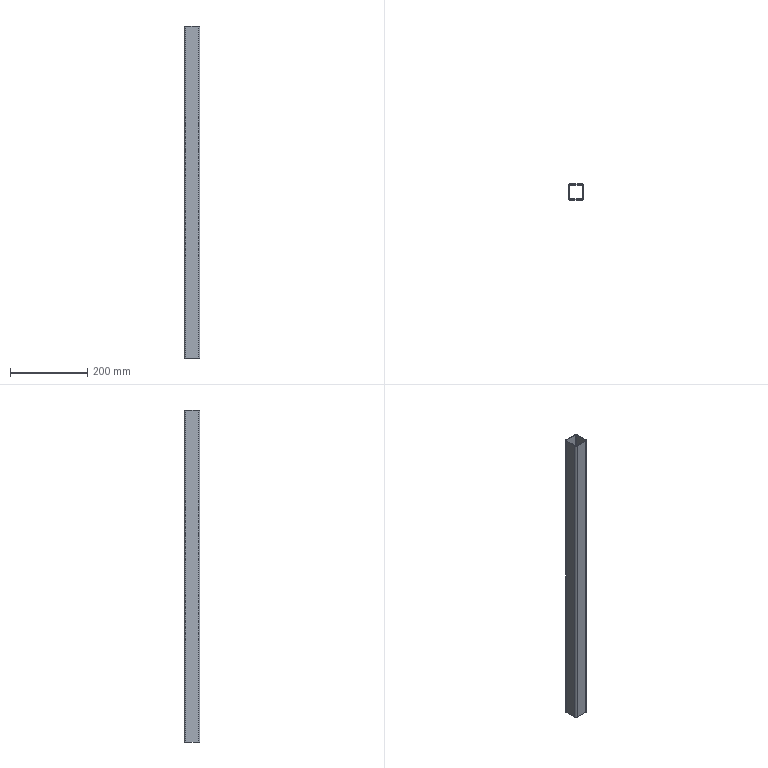Part | SolidWorks | features Fillet 2, Extrusion 1 | 1 solid | 18 faces | box 40 x 40 x 860 mm | volume 252581 mm3 | plane 10 | cylinder 8 | commonest cylinder face diameters 4 x4 8 x4
STEP:
#1=CARTESIAN_POINT('',(20.,-16.,860.));
#2=VERTEX_POINT('',#1);
#3=CARTESIAN_POINT('',(20.,16.,860.));
#4=VERTEX_POINT('',#3);
#5=CARTESIAN_POINT('',(20.,20.,860.));
#6=DIRECTION('',(0.,1.,0.));
#7=VECTOR('',#6,1000.);
#8=LINE('',#5,#7);
#9=EDGE_CURVE('',#2,#4,#8,.T.);
#10=ORIENTED_EDGE('',*,*,#9,.T.);
#11=CARTESIAN_POINT('',(16.,20.,860.));
#12=VERTEX_POINT('',#11);
#13=CARTESIAN_POINT('',(16.,16.,860.));
#14=DIRECTION('',(0.,0.,1.));
#15=DIRECTION('',(1.,0.,0.));
#16=AXIS2_PLACEMENT_3D('',#13,#14,#15);
#17=CIRCLE('',#16,4.);
#18=EDGE_CURVE('',#4,#12,#17,.T.);
#19=ORIENTED_EDGE('',*,*,#18,.T.);
#20=CARTESIAN_POINT('',(-16.,20.,860.));
#21=VERTEX_POINT('',#20);
#22=CARTESIAN_POINT('',(-20.,20.,860.));
#23=DIRECTION('',(-1.,0.,0.));
#24=VECTOR('',#23,1000.);
#25=LINE('',#22,#24);
#26=EDGE_CURVE('',#12,#21,#25,.T.);
#27=ORIENTED_EDGE('',*,*,#26,.T.);
#28=CARTESIAN_POINT('',(-20.,16.,860.));
#29=VERTEX_POINT('',#28);
#30=CARTESIAN_POINT('',(-16.,16.,860.));
#31=DIRECTION('',(0.,0.,1.));
#32=DIRECTION('',(1.,0.,0.));
#33=AXIS2_PLACEMENT_3D('',#30,#31,#32);
#34=CIRCLE('',#33,4.);
#35=EDGE_CURVE('',#21,#29,#34,.T.);
#36=ORIENTED_EDGE('',*,*,#35,.T.);
#37=CARTESIAN_POINT('',(-20.,-16.,860.));
#38=VERTEX_POINT('',#37);
#39=CARTESIAN_POINT('',(-20.,20.,860.));
#40=DIRECTION('',(0.,-1.,0.));
#41=VECTOR('',#40,1000.);
#42=LINE('',#39,#41);
#43=EDGE_CURVE('',#29,#38,#42,.T.);
#44=ORIENTED_EDGE('',*,*,#43,.T.);
#45=CARTESIAN_POINT('',(-16.,-20.,860.));
#46=VERTEX_POINT('',#45);
#47=CARTESIAN_POINT('',(-16.,-16.,860.));
#48=DIRECTION('',(0.,0.,1.));
#49=DIRECTION('',(1.,0.,0.));
#50=AXIS2_PLACEMENT_3D('',#47,#48,#49);
#51=CIRCLE('',#50,4.);
#52=EDGE_CURVE('',#38,#46,#51,.T.);
#53=ORIENTED_EDGE('',*,*,#52,.T.);
#54=CARTESIAN_POINT('',(16.,-20.,860.));
#55=VERTEX_POINT('',#54);
#56=CARTESIAN_POINT('',(-20.,-20.,860.));
#57=DIRECTION('',(1.,0.,0.));
#58=VECTOR('',#57,1000.);
#59=LINE('',#56,#58);
#60=EDGE_CURVE('',#46,#55,#59,.T.);
#61=ORIENTED_EDGE('',*,*,#60,.T.);
#62=CARTESIAN_POINT('',(16.,-16.,860.));
#63=DIRECTION('',(0.,0.,1.));
#64=DIRECTION('',(1.,0.,0.));
#65=AXIS2_PLACEMENT_3D('',#62,#63,#64);
#66=CIRCLE('',#65,4.);
#67=EDGE_CURVE('',#55,#2,#66,.T.);
#68=ORIENTED_EDGE('',*,*,#67,.T.);
#69=EDGE_LOOP('',(#10,#19,#27,#36,#44,#53,#61,#68));
#70=FACE_OUTER_BOUND('',#69,.T.);
#71=CARTESIAN_POINT('',(16.,18.,860.));
#72=VERTEX_POINT('',#71);
#73=CARTESIAN_POINT('',(-16.,18.,860.));
#74=VERTEX_POINT('',#73);
#75=CARTESIAN_POINT('',(-18.,18.,860.));
#76=DIRECTION('',(-1.,0.,0.));
#77=VECTOR('',#76,1000.);
#78=LINE('',#75,#77);
#79=EDGE_CURVE('',#72,#74,#78,.T.);
#80=ORIENTED_EDGE('',*,*,#79,.F.);
#81=CARTESIAN_POINT('',(18.,16.,860.));
#82=VERTEX_POINT('',#81);
#83=CARTESIAN_POINT('',(16.,16.,860.));
#84=DIRECTION('',(0.,0.,-1.));
#85=DIRECTION('',(1.,0.,0.));
#86=AXIS2_PLACEMENT_3D('',#83,#84,#85);
#87=CIRCLE('',#86,2.);
#88=EDGE_CURVE('',#72,#82,#87,.T.);
#89=ORIENTED_EDGE('',*,*,#88,.T.);
#90=CARTESIAN_POINT('',(18.,-16.,860.));
#91=VERTEX_POINT('',#90);
#92=CARTESIAN_POINT('',(18.,18.,860.));
#93=DIRECTION('',(0.,1.,0.));
#94=VECTOR('',#93,1000.);
#95=LINE('',#92,#94);
#96=EDGE_CURVE('',#91,#82,#95,.T.);
#97=ORIENTED_EDGE('',*,*,#96,.F.);
#98=CARTESIAN_POINT('',(16.,-18.,860.));
#99=VERTEX_POINT('',#98);
#100=CARTESIAN_POINT('',(16.,-16.,860.));
#101=DIRECTION('',(0.,0.,-1.));
#102=DIRECTION('',(1.,0.,0.));
#103=AXIS2_PLACEMENT_3D('',#100,#101,#102);
#104=CIRCLE('',#103,2.);
#105=EDGE_CURVE('',#91,#99,#104,.T.);
#106=ORIENTED_EDGE('',*,*,#105,.T.);
#107=CARTESIAN_POINT('',(-16.,-18.,860.));
#108=VERTEX_POINT('',#107);
#109=CARTESIAN_POINT('',(-18.,-18.,860.));
#110=DIRECTION('',(1.,0.,0.));
#111=VECTOR('',#110,1000.);
#112=LINE('',#109,#111);
#113=EDGE_CURVE('',#108,#99,#112,.T.);
#114=ORIENTED_EDGE('',*,*,#113,.F.);
#115=CARTESIAN_POINT('',(-18.,-16.,860.));
#116=VERTEX_POINT('',#115);
#117=CARTESIAN_POINT('',(-16.,-16.,860.));
#118=DIRECTION('',(0.,0.,-1.));
#119=DIRECTION('',(1.,0.,0.));
#120=AXIS2_PLACEMENT_3D('',#117,#118,#119);
#121=CIRCLE('',#120,2.);
#122=EDGE_CURVE('',#108,#116,#121,.T.);
#123=ORIENTED_EDGE('',*,*,#122,.T.);
#124=CARTESIAN_POINT('',(-18.,16.,860.));
#125=VERTEX_POINT('',#124);
#126=CARTESIAN_POINT('',(-18.,18.,860.));
#127=DIRECTION('',(0.,-1.,0.));
#128=VECTOR('',#127,1000.);
#129=LINE('',#126,#128);
#130=EDGE_CURVE('',#125,#116,#129,.T.);
#131=ORIENTED_EDGE('',*,*,#130,.F.);
#132=CARTESIAN_POINT('',(-16.,16.,860.));
#133=DIRECTION('',(0.,0.,-1.));
#134=DIRECTION('',(1.,0.,0.));
#135=AXIS2_PLACEMENT_3D('',#132,#133,#134);
#136=CIRCLE('',#135,2.);
#137=EDGE_CURVE('',#125,#74,#136,.T.);
#138=ORIENTED_EDGE('',*,*,#137,.T.);
#139=EDGE_LOOP('',(#80,#89,#97,#106,#114,#123,#131,#138));
#140=FACE_BOUND('',#139,.T.);
#141=CARTESIAN_POINT('',(0.,0.,860.));
#142=DIRECTION('',(0.,0.,1.));
#143=DIRECTION('',(1.,0.,0.));
#144=AXIS2_PLACEMENT_3D('',#141,#142,#143);
#145=PLANE('',#144);
#146=ADVANCED_FACE('',(#70,#140),#145,.T.);
#147=CARTESIAN_POINT('',(16.,20.,0.));
#148=VERTEX_POINT('',#147);
#149=CARTESIAN_POINT('',(-16.,20.,0.));
#150=VERTEX_POINT('',#149);
#151=CARTESIAN_POINT('',(-20.,20.,0.));
#152=DIRECTION('',(-1.,0.,0.));
#153=VECTOR('',#152,1000.);
#154=LINE('',#151,#153);
#155=EDGE_CURVE('',#148,#150,#154,.T.);
#156=ORIENTED_EDGE('',*,*,#155,.F.);
#157=CARTESIAN_POINT('',(20.,16.,0.));
#158=VERTEX_POINT('',#157);
#159=CARTESIAN_POINT('',(16.,16.,0.));
#160=DIRECTION('',(0.,0.,-1.));
#161=DIRECTION('',(1.,0.,0.));
#162=AXIS2_PLACEMENT_3D('',#159,#160,#161);
#163=CIRCLE('',#162,4.);
#164=EDGE_CURVE('',#148,#158,#163,.T.);
#165=ORIENTED_EDGE('',*,*,#164,.T.);
#166=CARTESIAN_POINT('',(20.,-16.,0.));
#167=VERTEX_POINT('',#166);
#168=CARTESIAN_POINT('',(20.,20.,0.));
#169=DIRECTION('',(0.,1.,0.));
#170=VECTOR('',#169,1000.);
#171=LINE('',#168,#170);
#172=EDGE_CURVE('',#167,#158,#171,.T.);
#173=ORIENTED_EDGE('',*,*,#172,.F.);
#174=CARTESIAN_POINT('',(16.,-20.,0.));
#175=VERTEX_POINT('',#174);
#176=CARTESIAN_POINT('',(16.,-16.,0.));
#177=DIRECTION('',(0.,0.,-1.));
#178=DIRECTION('',(1.,0.,0.));
#179=AXIS2_PLACEMENT_3D('',#176,#177,#178);
#180=CIRCLE('',#179,4.);
#181=EDGE_CURVE('',#167,#175,#180,.T.);
#182=ORIENTED_EDGE('',*,*,#181,.T.);
#183=CARTESIAN_POINT('',(-16.,-20.,0.));
#184=VERTEX_POINT('',#183);
#185=CARTESIAN_POINT('',(-20.,-20.,0.));
#186=DIRECTION('',(1.,0.,0.));
#187=VECTOR('',#186,1000.);
#188=LINE('',#185,#187);
#189=EDGE_CURVE('',#184,#175,#188,.T.);
#190=ORIENTED_EDGE('',*,*,#189,.F.);
#191=CARTESIAN_POINT('',(-20.,-16.,0.));
#192=VERTEX_POINT('',#191);
#193=CARTESIAN_POINT('',(-16.,-16.,0.));
#194=DIRECTION('',(0.,0.,-1.));
#195=DIRECTION('',(1.,0.,0.));
#196=AXIS2_PLACEMENT_3D('',#193,#194,#195);
#197=CIRCLE('',#196,4.);
#198=EDGE_CURVE('',#184,#192,#197,.T.);
#199=ORIENTED_EDGE('',*,*,#198,.T.);
#200=CARTESIAN_POINT('',(-20.,16.,0.));
#201=VERTEX_POINT('',#200);
#202=CARTESIAN_POINT('',(-20.,20.,0.));
#203=DIRECTION('',(0.,-1.,0.));
#204=VECTOR('',#203,1000.);
#205=LINE('',#202,#204);
#206=EDGE_CURVE('',#201,#192,#205,.T.);
#207=ORIENTED_EDGE('',*,*,#206,.F.);
#208=CARTESIAN_POINT('',(-16.,16.,0.));
#209=DIRECTION('',(0.,0.,-1.));
#210=DIRECTION('',(1.,0.,0.));
#211=AXIS2_PLACEMENT_3D('',#208,#209,#210);
#212=CIRCLE('',#211,4.);
#213=EDGE_CURVE('',#201,#150,#212,.T.);
#214=ORIENTED_EDGE('',*,*,#213,.T.);
#215=EDGE_LOOP('',(#156,#165,#173,#182,#190,#199,#207,#214));
#216=FACE_OUTER_BOUND('',#215,.T.);
#217=CARTESIAN_POINT('',(-16.,-18.,0.));
#218=VERTEX_POINT('',#217);
#219=CARTESIAN_POINT('',(16.,-18.,0.));
#220=VERTEX_POINT('',#219);
#221=CARTESIAN_POINT('',(-18.,-18.,0.));
#222=DIRECTION('',(1.,0.,0.));
#223=VECTOR('',#222,1000.);
#224=LINE('',#221,#223);
#225=EDGE_CURVE('',#218,#220,#224,.T.);
#226=ORIENTED_EDGE('',*,*,#225,.T.);
#227=CARTESIAN_POINT('',(18.,-16.,0.));
#228=VERTEX_POINT('',#227);
#229=CARTESIAN_POINT('',(16.,-16.,0.));
#230=DIRECTION('',(0.,0.,1.));
#231=DIRECTION('',(1.,0.,0.));
#232=AXIS2_PLACEMENT_3D('',#229,#230,#231);
#233=CIRCLE('',#232,2.);
#234=EDGE_CURVE('',#220,#228,#233,.T.);
#235=ORIENTED_EDGE('',*,*,#234,.T.);
#236=CARTESIAN_POINT('',(18.,16.,0.));
#237=VERTEX_POINT('',#236);
#238=CARTESIAN_POINT('',(18.,18.,0.));
#239=DIRECTION('',(0.,1.,0.));
#240=VECTOR('',#239,1000.);
#241=LINE('',#238,#240);
#242=EDGE_CURVE('',#228,#237,#241,.T.);
#243=ORIENTED_EDGE('',*,*,#242,.T.);
#244=CARTESIAN_POINT('',(16.,18.,0.));
#245=VERTEX_POINT('',#244);
#246=CARTESIAN_POINT('',(16.,16.,0.));
#247=DIRECTION('',(0.,0.,1.));
#248=DIRECTION('',(1.,0.,0.));
#249=AXIS2_PLACEMENT_3D('',#246,#247,#248);
#250=CIRCLE('',#249,2.);
#251=EDGE_CURVE('',#237,#245,#250,.T.);
#252=ORIENTED_EDGE('',*,*,#251,.T.);
#253=CARTESIAN_POINT('',(-16.,18.,0.));
#254=VERTEX_POINT('',#253);
#255=CARTESIAN_POINT('',(-18.,18.,0.));
#256=DIRECTION('',(-1.,0.,0.));
#257=VECTOR('',#256,1000.);
#258=LINE('',#255,#257);
#259=EDGE_CURVE('',#245,#254,#258,.T.);
#260=ORIENTED_EDGE('',*,*,#259,.T.);
#261=CARTESIAN_POINT('',(-18.,16.,0.));
#262=VERTEX_POINT('',#261);
#263=CARTESIAN_POINT('',(-16.,16.,0.));
#264=DIRECTION('',(0.,0.,1.));
#265=DIRECTION('',(1.,0.,0.));
#266=AXIS2_PLACEMENT_3D('',#263,#264,#265);
#267=CIRCLE('',#266,2.);
#268=EDGE_CURVE('',#254,#262,#267,.T.);
#269=ORIENTED_EDGE('',*,*,#268,.T.);
#270=CARTESIAN_POINT('',(-18.,-16.,0.));
#271=VERTEX_POINT('',#270);
#272=CARTESIAN_POINT('',(-18.,18.,0.));
#273=DIRECTION('',(0.,-1.,0.));
#274=VECTOR('',#273,1000.);
#275=LINE('',#272,#274);
#276=EDGE_CURVE('',#262,#271,#275,.T.);
#277=ORIENTED_EDGE('',*,*,#276,.T.);
#278=CARTESIAN_POINT('',(-16.,-16.,0.));
#279=DIRECTION('',(0.,0.,1.));
#280=DIRECTION('',(1.,0.,0.));
#281=AXIS2_PLACEMENT_3D('',#278,#279,#280);
#282=CIRCLE('',#281,2.);
#283=EDGE_CURVE('',#271,#218,#282,.T.);
#284=ORIENTED_EDGE('',*,*,#283,.T.);
#285=EDGE_LOOP('',(#226,#235,#243,#252,#260,#269,#277,#284));
#286=FACE_BOUND('',#285,.T.);
#287=CARTESIAN_POINT('',(0.,0.,0.));
#288=DIRECTION('',(0.,0.,1.));
#289=DIRECTION('',(1.,0.,0.));
#290=AXIS2_PLACEMENT_3D('',#287,#288,#289);
#291=PLANE('',#290);
#292=ADVANCED_FACE('',(#216,#286),#291,.F.);
#293=ORIENTED_EDGE('',*,*,#172,.T.);
#294=CARTESIAN_POINT('',(20.,16.,860.));
#295=DIRECTION('',(0.,0.,1.));
#296=VECTOR('',#295,1000.);
#297=LINE('',#294,#296);
#298=EDGE_CURVE('',#158,#4,#297,.T.);
#299=ORIENTED_EDGE('',*,*,#298,.T.);
#300=ORIENTED_EDGE('',*,*,#9,.F.);
#301=CARTESIAN_POINT('',(20.,-16.,860.));
#302=DIRECTION('',(0.,0.,-1.));
#303=VECTOR('',#302,1000.);
#304=LINE('',#301,#303);
#305=EDGE_CURVE('',#2,#167,#304,.T.);
#306=ORIENTED_EDGE('',*,*,#305,.T.);
#307=EDGE_LOOP('',(#293,#299,#300,#306));
#308=FACE_OUTER_BOUND('',#307,.T.);
#309=CARTESIAN_POINT('',(20.,20.,860.));
#310=DIRECTION('',(-1.,0.,0.));
#311=DIRECTION('',(0.,0.,1.));
#312=AXIS2_PLACEMENT_3D('',#309,#310,#311);
#313=PLANE('',#312);
#314=ADVANCED_FACE('',(#308),#313,.F.);
#315=ORIENTED_EDGE('',*,*,#26,.F.);
#316=CARTESIAN_POINT('',(16.,20.,860.));
#317=DIRECTION('',(0.,0.,-1.));
#318=VECTOR('',#317,1000.);
#319=LINE('',#316,#318);
#320=EDGE_CURVE('',#12,#148,#319,.T.);
#321=ORIENTED_EDGE('',*,*,#320,.T.);
#322=ORIENTED_EDGE('',*,*,#155,.T.);
#323=CARTESIAN_POINT('',(-16.,20.,860.));
#324=DIRECTION('',(0.,0.,1.));
#325=VECTOR('',#324,1000.);
#326=LINE('',#323,#325);
#327=EDGE_CURVE('',#150,#21,#326,.T.);
#328=ORIENTED_EDGE('',*,*,#327,.T.);
#329=EDGE_LOOP('',(#315,#321,#322,#328));
#330=FACE_OUTER_BOUND('',#329,.T.);
#331=CARTESIAN_POINT('',(-20.,20.,860.));
#332=DIRECTION('',(0.,-1.,0.));
#333=DIRECTION('',(0.,0.,-1.));
#334=AXIS2_PLACEMENT_3D('',#331,#332,#333);
#335=PLANE('',#334);
#336=ADVANCED_FACE('',(#330),#335,.F.);
#337=ORIENTED_EDGE('',*,*,#43,.F.);
#338=CARTESIAN_POINT('',(-20.,16.,860.));
#339=DIRECTION('',(0.,0.,-1.));
#340=VECTOR('',#339,1000.);
#341=LINE('',#338,#340);
#342=EDGE_CURVE('',#29,#201,#341,.T.);
#343=ORIENTED_EDGE('',*,*,#342,.T.);
#344=ORIENTED_EDGE('',*,*,#206,.T.);
#345=CARTESIAN_POINT('',(-20.,-16.,860.));
#346=DIRECTION('',(0.,0.,1.));
#347=VECTOR('',#346,1000.);
#348=LINE('',#345,#347);
#349=EDGE_CURVE('',#192,#38,#348,.T.);
#350=ORIENTED_EDGE('',*,*,#349,.T.);
#351=EDGE_LOOP('',(#337,#343,#344,#350));
#352=FACE_OUTER_BOUND('',#351,.T.);
#353=CARTESIAN_POINT('',(-20.,20.,860.));
#354=DIRECTION('',(1.,0.,0.));
#355=DIRECTION('',(0.,0.,-1.));
#356=AXIS2_PLACEMENT_3D('',#353,#354,#355);
#357=PLANE('',#356);
#358=ADVANCED_FACE('',(#352),#357,.F.);
#359=ORIENTED_EDGE('',*,*,#189,.T.);
#360=CARTESIAN_POINT('',(16.,-20.,860.));
#361=DIRECTION('',(0.,0.,1.));
#362=VECTOR('',#361,1000.);
#363=LINE('',#360,#362);
#364=EDGE_CURVE('',#175,#55,#363,.T.);
#365=ORIENTED_EDGE('',*,*,#364,.T.);
#366=ORIENTED_EDGE('',*,*,#60,.F.);
#367=CARTESIAN_POINT('',(-16.,-20.,860.));
#368=DIRECTION('',(0.,0.,-1.));
#369=VECTOR('',#368,1000.);
#370=LINE('',#367,#369);
#371=EDGE_CURVE('',#46,#184,#370,.T.);
#372=ORIENTED_EDGE('',*,*,#371,.T.);
#373=EDGE_LOOP('',(#359,#365,#366,#372));
#374=FACE_OUTER_BOUND('',#373,.T.);
#375=CARTESIAN_POINT('',(-20.,-20.,860.));
#376=DIRECTION('',(0.,1.,0.));
#377=DIRECTION('',(0.,0.,1.));
#378=AXIS2_PLACEMENT_3D('',#375,#376,#377);
#379=PLANE('',#378);
#380=ADVANCED_FACE('',(#374),#379,.F.);
#381=ORIENTED_EDGE('',*,*,#96,.T.);
#382=CARTESIAN_POINT('',(18.,16.,0.));
#383=DIRECTION('',(0.,0.,-1.));
#384=VECTOR('',#383,1000.);
#385=LINE('',#382,#384);
#386=EDGE_CURVE('',#82,#237,#385,.T.);
#387=ORIENTED_EDGE('',*,*,#386,.T.);
#388=ORIENTED_EDGE('',*,*,#242,.F.);
#389=CARTESIAN_POINT('',(18.,-16.,860.));
#390=DIRECTION('',(0.,0.,1.));
#391=VECTOR('',#390,1000.);
#392=LINE('',#389,#391);
#393=EDGE_CURVE('',#228,#91,#392,.T.);
#394=ORIENTED_EDGE('',*,*,#393,.T.);
#395=EDGE_LOOP('',(#381,#387,#388,#394));
#396=FACE_OUTER_BOUND('',#395,.T.);
#397=CARTESIAN_POINT('',(18.,18.,860.));
#398=DIRECTION('',(-1.,0.,0.));
#399=DIRECTION('',(0.,0.,1.));
#400=AXIS2_PLACEMENT_3D('',#397,#398,#399);
#401=PLANE('',#400);
#402=ADVANCED_FACE('',(#396),#401,.T.);
#403=ORIENTED_EDGE('',*,*,#259,.F.);
#404=CARTESIAN_POINT('',(16.,18.,860.));
#405=DIRECTION('',(0.,0.,1.));
#406=VECTOR('',#405,1000.);
#407=LINE('',#404,#406);
#408=EDGE_CURVE('',#245,#72,#407,.T.);
#409=ORIENTED_EDGE('',*,*,#408,.T.);
#410=ORIENTED_EDGE('',*,*,#79,.T.);
#411=CARTESIAN_POINT('',(-16.,18.,0.));
#412=DIRECTION('',(0.,0.,-1.));
#413=VECTOR('',#412,1000.);
#414=LINE('',#411,#413);
#415=EDGE_CURVE('',#74,#254,#414,.T.);
#416=ORIENTED_EDGE('',*,*,#415,.T.);
#417=EDGE_LOOP('',(#403,#409,#410,#416));
#418=FACE_OUTER_BOUND('',#417,.T.);
#419=CARTESIAN_POINT('',(-18.,18.,860.));
#420=DIRECTION('',(0.,-1.,0.));
#421=DIRECTION('',(0.,0.,-1.));
#422=AXIS2_PLACEMENT_3D('',#419,#420,#421);
#423=PLANE('',#422);
#424=ADVANCED_FACE('',(#418),#423,.T.);
#425=ORIENTED_EDGE('',*,*,#276,.F.);
#426=CARTESIAN_POINT('',(-18.,16.,860.));
#427=DIRECTION('',(0.,0.,1.));
#428=VECTOR('',#427,1000.);
#429=LINE('',#426,#428);
#430=EDGE_CURVE('',#262,#125,#429,.T.);
#431=ORIENTED_EDGE('',*,*,#430,.T.);
#432=ORIENTED_EDGE('',*,*,#130,.T.);
#433=CARTESIAN_POINT('',(-18.,-16.,0.));
#434=DIRECTION('',(0.,0.,-1.));
#435=VECTOR('',#434,1000.);
#436=LINE('',#433,#435);
#437=EDGE_CURVE('',#116,#271,#436,.T.);
#438=ORIENTED_EDGE('',*,*,#437,.T.);
#439=EDGE_LOOP('',(#425,#431,#432,#438));
#440=FACE_OUTER_BOUND('',#439,.T.);
#441=CARTESIAN_POINT('',(-18.,18.,860.));
#442=DIRECTION('',(1.,0.,0.));
#443=DIRECTION('',(0.,0.,-1.));
#444=AXIS2_PLACEMENT_3D('',#441,#442,#443);
#445=PLANE('',#444);
#446=ADVANCED_FACE('',(#440),#445,.T.);
#447=ORIENTED_EDGE('',*,*,#225,.F.);
#448=CARTESIAN_POINT('',(-16.,-18.,860.));
#449=DIRECTION('',(0.,0.,1.));
#450=VECTOR('',#449,1000.);
#451=LINE('',#448,#450);
#452=EDGE_CURVE('',#218,#108,#451,.T.);
#453=ORIENTED_EDGE('',*,*,#452,.T.);
#454=ORIENTED_EDGE('',*,*,#113,.T.);
#455=CARTESIAN_POINT('',(16.,-18.,0.));
#456=DIRECTION('',(0.,0.,-1.));
#457=VECTOR('',#456,1000.);
#458=LINE('',#455,#457);
#459=EDGE_CURVE('',#99,#220,#458,.T.);
#460=ORIENTED_EDGE('',*,*,#459,.T.);
#461=EDGE_LOOP('',(#447,#453,#454,#460));
#462=FACE_OUTER_BOUND('',#461,.T.);
#463=CARTESIAN_POINT('',(-18.,-18.,860.));
#464=DIRECTION('',(0.,1.,0.));
#465=DIRECTION('',(0.,0.,1.));
#466=AXIS2_PLACEMENT_3D('',#463,#464,#465);
#467=PLANE('',#466);
#468=ADVANCED_FACE('',(#462),#467,.T.);
#469=ORIENTED_EDGE('',*,*,#88,.F.);
#470=ORIENTED_EDGE('',*,*,#408,.F.);
#471=ORIENTED_EDGE('',*,*,#251,.F.);
#472=ORIENTED_EDGE('',*,*,#386,.F.);
#473=EDGE_LOOP('',(#469,#470,#471,#472));
#474=FACE_OUTER_BOUND('',#473,.T.);
#475=CARTESIAN_POINT('',(16.,16.,860.));
#476=DIRECTION('',(0.,0.,1.));
#477=DIRECTION('',(1.,0.,0.));
#478=AXIS2_PLACEMENT_3D('',#475,#476,#477);
#479=CYLINDRICAL_SURFACE('',#478,2.);
#480=ADVANCED_FACE('',(#474),#479,.F.);
#481=ORIENTED_EDGE('',*,*,#137,.F.);
#482=ORIENTED_EDGE('',*,*,#430,.F.);
#483=ORIENTED_EDGE('',*,*,#268,.F.);
#484=ORIENTED_EDGE('',*,*,#415,.F.);
#485=EDGE_LOOP('',(#481,#482,#483,#484));
#486=FACE_OUTER_BOUND('',#485,.T.);
#487=CARTESIAN_POINT('',(-16.,16.,860.));
#488=DIRECTION('',(0.,0.,1.));
#489=DIRECTION('',(1.,0.,0.));
#490=AXIS2_PLACEMENT_3D('',#487,#488,#489);
#491=CYLINDRICAL_SURFACE('',#490,2.);
#492=ADVANCED_FACE('',(#486),#491,.F.);
#493=ORIENTED_EDGE('',*,*,#122,.F.);
#494=ORIENTED_EDGE('',*,*,#452,.F.);
#495=ORIENTED_EDGE('',*,*,#283,.F.);
#496=ORIENTED_EDGE('',*,*,#437,.F.);
#497=EDGE_LOOP('',(#493,#494,#495,#496));
#498=FACE_OUTER_BOUND('',#497,.T.);
#499=CARTESIAN_POINT('',(-16.,-16.,860.));
#500=DIRECTION('',(0.,0.,1.));
#501=DIRECTION('',(1.,0.,0.));
#502=AXIS2_PLACEMENT_3D('',#499,#500,#501);
#503=CYLINDRICAL_SURFACE('',#502,2.);
#504=ADVANCED_FACE('',(#498),#503,.F.);
#505=ORIENTED_EDGE('',*,*,#105,.F.);
#506=ORIENTED_EDGE('',*,*,#393,.F.);
#507=ORIENTED_EDGE('',*,*,#234,.F.);
#508=ORIENTED_EDGE('',*,*,#459,.F.);
#509=EDGE_LOOP('',(#505,#506,#507,#508));
#510=FACE_OUTER_BOUND('',#509,.T.);
#511=CARTESIAN_POINT('',(16.,-16.,860.));
#512=DIRECTION('',(0.,0.,1.));
#513=DIRECTION('',(1.,0.,0.));
#514=AXIS2_PLACEMENT_3D('',#511,#512,#513);
#515=CYLINDRICAL_SURFACE('',#514,2.);
#516=ADVANCED_FACE('',(#510),#515,.F.);
#517=ORIENTED_EDGE('',*,*,#18,.F.);
#518=ORIENTED_EDGE('',*,*,#298,.F.);
#519=ORIENTED_EDGE('',*,*,#164,.F.);
#520=ORIENTED_EDGE('',*,*,#320,.F.);
#521=EDGE_LOOP('',(#517,#518,#519,#520));
#522=FACE_OUTER_BOUND('',#521,.T.);
#523=CARTESIAN_POINT('',(16.,16.,860.));
#524=DIRECTION('',(0.,0.,-1.));
#525=DIRECTION('',(-1.,0.,0.));
#526=AXIS2_PLACEMENT_3D('',#523,#524,#525);
#527=CYLINDRICAL_SURFACE('',#526,4.);
#528=ADVANCED_FACE('',(#522),#527,.T.);
#529=ORIENTED_EDGE('',*,*,#67,.F.);
#530=ORIENTED_EDGE('',*,*,#364,.F.);
#531=ORIENTED_EDGE('',*,*,#181,.F.);
#532=ORIENTED_EDGE('',*,*,#305,.F.);
#533=EDGE_LOOP('',(#529,#530,#531,#532));
#534=FACE_OUTER_BOUND('',#533,.T.);
#535=CARTESIAN_POINT('',(16.,-16.,860.));
#536=DIRECTION('',(0.,0.,-1.));
#537=DIRECTION('',(-1.,0.,0.));
#538=AXIS2_PLACEMENT_3D('',#535,#536,#537);
#539=CYLINDRICAL_SURFACE('',#538,4.);
#540=ADVANCED_FACE('',(#534),#539,.T.);
#541=ORIENTED_EDGE('',*,*,#35,.F.);
#542=ORIENTED_EDGE('',*,*,#327,.F.);
#543=ORIENTED_EDGE('',*,*,#213,.F.);
#544=ORIENTED_EDGE('',*,*,#342,.F.);
#545=EDGE_LOOP('',(#541,#542,#543,#544));
#546=FACE_OUTER_BOUND('',#545,.T.);
#547=CARTESIAN_POINT('',(-16.,16.,860.));
#548=DIRECTION('',(0.,0.,-1.));
#549=DIRECTION('',(-1.,0.,0.));
#550=AXIS2_PLACEMENT_3D('',#547,#548,#549);
#551=CYLINDRICAL_SURFACE('',#550,4.);
#552=ADVANCED_FACE('',(#546),#551,.T.);
#553=ORIENTED_EDGE('',*,*,#52,.F.);
#554=ORIENTED_EDGE('',*,*,#349,.F.);
#555=ORIENTED_EDGE('',*,*,#198,.F.);
#556=ORIENTED_EDGE('',*,*,#371,.F.);
#557=EDGE_LOOP('',(#553,#554,#555,#556));
#558=FACE_OUTER_BOUND('',#557,.T.);
#559=CARTESIAN_POINT('',(-16.,-16.,860.));
#560=DIRECTION('',(0.,0.,-1.));
#561=DIRECTION('',(-1.,0.,0.));
#562=AXIS2_PLACEMENT_3D('',#559,#560,#561);
#563=CYLINDRICAL_SURFACE('',#562,4.);
#564=ADVANCED_FACE('',(#558),#563,.T.);
#565=CLOSED_SHELL('',(#146,#292,#314,#336,#358,#380,#402,#424,#446,#468,#480,#492,#504,#516,#528,#540,#552,#564));
#566=MANIFOLD_SOLID_BREP('',#565);
#567=CARTESIAN_POINT('',(0.,0.,0.));
#568=DIRECTION('',(0.,0.,1.));
#569=DIRECTION('',(1.,0.,0.));
#570=AXIS2_PLACEMENT_3D('',#567,#568,#569);
#571=(LENGTH_UNIT()NAMED_UNIT(*)SI_UNIT(.MILLI.,.METRE.));
#572=UNCERTAINTY_MEASURE_WITH_UNIT(LENGTH_MEASURE(0.00001),#571,'','');
#573=(NAMED_UNIT(*)PLANE_ANGLE_UNIT()SI_UNIT($,.RADIAN.));
#574=(NAMED_UNIT(*)SI_UNIT($,.STERADIAN.)SOLID_ANGLE_UNIT());
#575=(GEOMETRIC_REPRESENTATION_CONTEXT(3)GLOBAL_UNCERTAINTY_ASSIGNED_CONTEXT((#572))GLOBAL_UNIT_ASSIGNED_CONTEXT((#571,#573,#574))REPRESENTATION_CONTEXT('',''));
#576=ADVANCED_BREP_SHAPE_REPRESENTATION('',(#566,#570),#575);